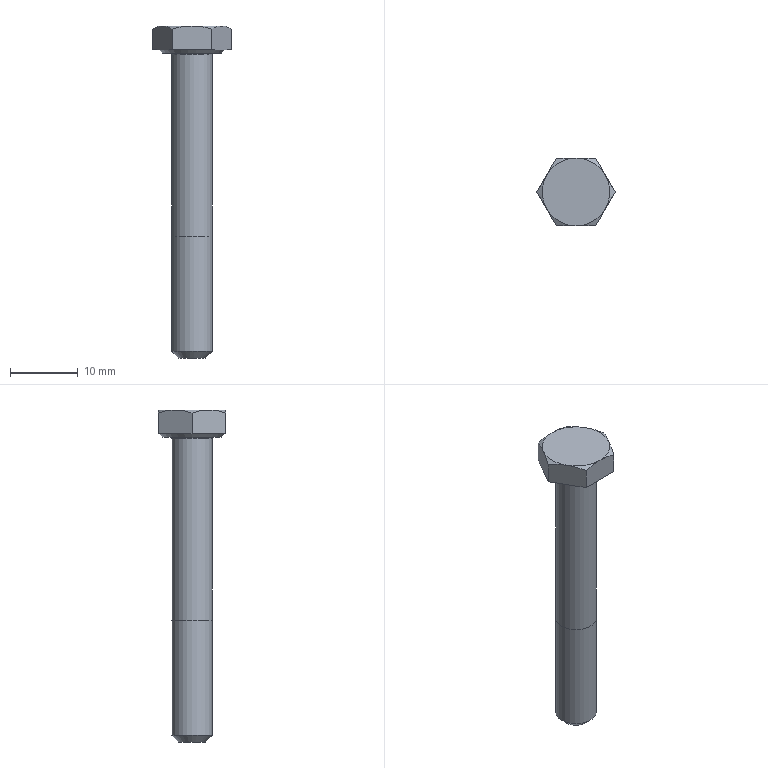Part | NX | features BREP 1, DATUM_CSYS 1 | 1 solid | 21 faces | box 11.547 x 10 x 49 mm | volume 1599 mm3 | plane 10 | cone 8 | cylinder 2 | torus 1 | commonest cylinder face diameters 6 x2
STEP:
#1=CARTESIAN_POINT('',(4.33,2.5,4.));
#2=VERTEX_POINT('',#1);
#3=CARTESIAN_POINT('',(4.33,-2.5,4.));
#4=VERTEX_POINT('',#3);
#5=CARTESIAN_POINT('',(0.,0.,4.));
#6=DIRECTION('',(0.,0.,-1.));
#7=DIRECTION('',(0.866,0.5,0.));
#8=AXIS2_PLACEMENT_3D('',#5,#6,#7);
#9=CIRCLE('',#8,5.);
#10=EDGE_CURVE('',#2,#4,#9,.T.);
#11=ORIENTED_EDGE('',*,*,#10,.F.);
#12=CARTESIAN_POINT('',(0.,5.,4.));
#13=VERTEX_POINT('',#12);
#14=CARTESIAN_POINT('',(0.,0.,4.));
#15=DIRECTION('',(0.,0.,1.));
#16=DIRECTION('',(0.866,0.5,0.));
#17=AXIS2_PLACEMENT_3D('',#14,#15,#16);
#18=CIRCLE('',#17,5.);
#19=EDGE_CURVE('',#2,#13,#18,.T.);
#20=ORIENTED_EDGE('',*,*,#19,.T.);
#21=CARTESIAN_POINT('',(-4.33,2.5,4.));
#22=VERTEX_POINT('',#21);
#23=CARTESIAN_POINT('',(0.,0.,4.));
#24=DIRECTION('',(0.,0.,1.));
#25=DIRECTION('',(0.,1.,0.));
#26=AXIS2_PLACEMENT_3D('',#23,#24,#25);
#27=CIRCLE('',#26,5.);
#28=EDGE_CURVE('',#13,#22,#27,.T.);
#29=ORIENTED_EDGE('',*,*,#28,.T.);
#30=CARTESIAN_POINT('',(-4.33,-2.5,4.));
#31=VERTEX_POINT('',#30);
#32=CARTESIAN_POINT('',(0.,0.,4.));
#33=DIRECTION('',(0.,0.,1.));
#34=DIRECTION('',(-0.866,0.5,0.));
#35=AXIS2_PLACEMENT_3D('',#32,#33,#34);
#36=CIRCLE('',#35,5.);
#37=EDGE_CURVE('',#22,#31,#36,.T.);
#38=ORIENTED_EDGE('',*,*,#37,.T.);
#39=CARTESIAN_POINT('',(0.,-5.,4.));
#40=VERTEX_POINT('',#39);
#41=CARTESIAN_POINT('',(0.,0.,4.));
#42=DIRECTION('',(0.,0.,1.));
#43=DIRECTION('',(-0.866,-0.5,0.));
#44=AXIS2_PLACEMENT_3D('',#41,#42,#43);
#45=CIRCLE('',#44,5.);
#46=EDGE_CURVE('',#31,#40,#45,.T.);
#47=ORIENTED_EDGE('',*,*,#46,.T.);
#48=CARTESIAN_POINT('',(0.,0.,4.));
#49=DIRECTION('',(0.,0.,1.));
#50=DIRECTION('',(0.,-1.,0.));
#51=AXIS2_PLACEMENT_3D('',#48,#49,#50);
#52=CIRCLE('',#51,5.);
#53=EDGE_CURVE('',#40,#4,#52,.T.);
#54=ORIENTED_EDGE('',*,*,#53,.T.);
#55=EDGE_LOOP('',(#11,#20,#29,#38,#47,#54));
#56=FACE_BOUND('',#55,.T.);
#57=CARTESIAN_POINT('',(0.,0.7735,4.));
#58=DIRECTION('',(0.,0.,1.));
#59=DIRECTION('',(-1.,0.,0.));
#60=AXIS2_PLACEMENT_3D('',#57,#58,#59);
#61=PLANE('',#60);
#62=ADVANCED_FACE('',(#56),#61,.T.);
#63=CARTESIAN_POINT('',(5.774,0.,0.5));
#64=VERTEX_POINT('',#63);
#65=CARTESIAN_POINT('',(2.887,5.,0.5));
#66=VERTEX_POINT('',#65);
#67=CARTESIAN_POINT('',(5.774,0.,0.5));
#68=DIRECTION('',(-0.5,0.866,0.));
#69=VECTOR('',#68,1000.);
#70=LINE('',#67,#69);
#71=EDGE_CURVE('',#64,#66,#70,.T.);
#72=ORIENTED_EDGE('',*,*,#71,.T.);
#73=CARTESIAN_POINT('',(2.887,5.,3.553));
#74=VERTEX_POINT('',#73);
#75=CARTESIAN_POINT('',(2.887,5.,0.5));
#76=DIRECTION('',(0.,0.,1.));
#77=VECTOR('',#76,1000.);
#78=LINE('',#75,#77);
#79=EDGE_CURVE('',#66,#74,#78,.T.);
#80=ORIENTED_EDGE('',*,*,#79,.T.);
#81=CARTESIAN_POINT('',(4.33,2.5,4.));
#82=CARTESIAN_POINT('',(3.66,3.66,4.));
#83=CARTESIAN_POINT('',(2.887,5.,3.553));
#84=(BOUNDED_CURVE()B_SPLINE_CURVE(2,(#81,#82,#83),.UNSPECIFIED.,.F.,.F.)B_SPLINE_CURVE_WITH_KNOTS((3,3),(0.,1.),.PIECEWISE_BEZIER_KNOTS.)CURVE()GEOMETRIC_REPRESENTATION_ITEM()RATIONAL_B_SPLINE_CURVE((1.444,1.444,1.34))REPRESENTATION_ITEM(''));
#85=EDGE_CURVE('',#2,#74,#84,.T.);
#86=ORIENTED_EDGE('',*,*,#85,.F.);
#87=CARTESIAN_POINT('',(5.774,0.,3.553));
#88=VERTEX_POINT('',#87);
#89=CARTESIAN_POINT('',(5.774,0.,3.553));
#90=CARTESIAN_POINT('',(5.,1.34,4.));
#91=CARTESIAN_POINT('',(4.33,2.5,4.));
#92=(BOUNDED_CURVE()B_SPLINE_CURVE(2,(#89,#90,#91),.UNSPECIFIED.,.F.,.F.)B_SPLINE_CURVE_WITH_KNOTS((3,3),(0.,1.),.PIECEWISE_BEZIER_KNOTS.)CURVE()GEOMETRIC_REPRESENTATION_ITEM()RATIONAL_B_SPLINE_CURVE((1.34,1.444,1.444))REPRESENTATION_ITEM(''));
#93=EDGE_CURVE('',#88,#2,#92,.T.);
#94=ORIENTED_EDGE('',*,*,#93,.F.);
#95=CARTESIAN_POINT('',(5.774,0.,0.5));
#96=DIRECTION('',(0.,0.,1.));
#97=VECTOR('',#96,1000.);
#98=LINE('',#95,#97);
#99=EDGE_CURVE('',#64,#88,#98,.T.);
#100=ORIENTED_EDGE('',*,*,#99,.F.);
#101=EDGE_LOOP('',(#72,#80,#86,#94,#100));
#102=FACE_BOUND('',#101,.T.);
#103=CARTESIAN_POINT('',(4.33,2.5,2.25));
#104=DIRECTION('',(0.866,0.5,0.));
#105=DIRECTION('',(0.5,-0.866,0.));
#106=AXIS2_PLACEMENT_3D('',#103,#104,#105);
#107=PLANE('',#106);
#108=ADVANCED_FACE('',(#102),#107,.T.);
#109=CARTESIAN_POINT('',(-2.887,5.,0.5));
#110=VERTEX_POINT('',#109);
#111=CARTESIAN_POINT('',(2.887,5.,0.5));
#112=DIRECTION('',(-1.,0.,0.));
#113=VECTOR('',#112,1000.);
#114=LINE('',#111,#113);
#115=EDGE_CURVE('',#66,#110,#114,.T.);
#116=ORIENTED_EDGE('',*,*,#115,.T.);
#117=CARTESIAN_POINT('',(-2.887,5.,3.553));
#118=VERTEX_POINT('',#117);
#119=CARTESIAN_POINT('',(-2.887,5.,0.5));
#120=DIRECTION('',(0.,0.,1.));
#121=VECTOR('',#120,1000.);
#122=LINE('',#119,#121);
#123=EDGE_CURVE('',#110,#118,#122,.T.);
#124=ORIENTED_EDGE('',*,*,#123,.T.);
#125=CARTESIAN_POINT('',(0.,5.,4.));
#126=CARTESIAN_POINT('',(-1.34,5.,4.));
#127=CARTESIAN_POINT('',(-2.887,5.,3.553));
#128=(BOUNDED_CURVE()B_SPLINE_CURVE(2,(#125,#126,#127),.UNSPECIFIED.,.F.,.F.)B_SPLINE_CURVE_WITH_KNOTS((3,3),(0.,1.),.PIECEWISE_BEZIER_KNOTS.)CURVE()GEOMETRIC_REPRESENTATION_ITEM()RATIONAL_B_SPLINE_CURVE((1.444,1.444,1.34))REPRESENTATION_ITEM(''));
#129=EDGE_CURVE('',#13,#118,#128,.T.);
#130=ORIENTED_EDGE('',*,*,#129,.F.);
#131=CARTESIAN_POINT('',(2.887,5.,3.553));
#132=CARTESIAN_POINT('',(1.34,5.,4.));
#133=CARTESIAN_POINT('',(0.,5.,4.));
#134=(BOUNDED_CURVE()B_SPLINE_CURVE(2,(#131,#132,#133),.UNSPECIFIED.,.F.,.F.)B_SPLINE_CURVE_WITH_KNOTS((3,3),(0.,1.),.PIECEWISE_BEZIER_KNOTS.)CURVE()GEOMETRIC_REPRESENTATION_ITEM()RATIONAL_B_SPLINE_CURVE((1.34,1.444,1.444))REPRESENTATION_ITEM(''));
#135=EDGE_CURVE('',#74,#13,#134,.T.);
#136=ORIENTED_EDGE('',*,*,#135,.F.);
#137=ORIENTED_EDGE('',*,*,#79,.F.);
#138=EDGE_LOOP('',(#116,#124,#130,#136,#137));
#139=FACE_BOUND('',#138,.T.);
#140=CARTESIAN_POINT('',(0.,5.,2.25));
#141=DIRECTION('',(0.,1.,0.));
#142=DIRECTION('',(1.,0.,0.));
#143=AXIS2_PLACEMENT_3D('',#140,#141,#142);
#144=PLANE('',#143);
#145=ADVANCED_FACE('',(#139),#144,.T.);
#146=CARTESIAN_POINT('',(-5.774,0.,0.5));
#147=VERTEX_POINT('',#146);
#148=CARTESIAN_POINT('',(-2.887,5.,0.5));
#149=DIRECTION('',(-0.5,-0.866,0.));
#150=VECTOR('',#149,1000.);
#151=LINE('',#148,#150);
#152=EDGE_CURVE('',#110,#147,#151,.T.);
#153=ORIENTED_EDGE('',*,*,#152,.T.);
#154=CARTESIAN_POINT('',(-5.774,0.,3.553));
#155=VERTEX_POINT('',#154);
#156=CARTESIAN_POINT('',(-5.774,0.,0.5));
#157=DIRECTION('',(0.,0.,1.));
#158=VECTOR('',#157,1000.);
#159=LINE('',#156,#158);
#160=EDGE_CURVE('',#147,#155,#159,.T.);
#161=ORIENTED_EDGE('',*,*,#160,.T.);
#162=CARTESIAN_POINT('',(-4.33,2.5,4.));
#163=CARTESIAN_POINT('',(-5.,1.34,4.));
#164=CARTESIAN_POINT('',(-5.774,0.,3.553));
#165=(BOUNDED_CURVE()B_SPLINE_CURVE(2,(#162,#163,#164),.UNSPECIFIED.,.F.,.F.)B_SPLINE_CURVE_WITH_KNOTS((3,3),(0.,1.),.PIECEWISE_BEZIER_KNOTS.)CURVE()GEOMETRIC_REPRESENTATION_ITEM()RATIONAL_B_SPLINE_CURVE((1.444,1.444,1.34))REPRESENTATION_ITEM(''));
#166=EDGE_CURVE('',#22,#155,#165,.T.);
#167=ORIENTED_EDGE('',*,*,#166,.F.);
#168=CARTESIAN_POINT('',(-2.887,5.,3.553));
#169=CARTESIAN_POINT('',(-3.66,3.66,4.));
#170=CARTESIAN_POINT('',(-4.33,2.5,4.));
#171=(BOUNDED_CURVE()B_SPLINE_CURVE(2,(#168,#169,#170),.UNSPECIFIED.,.F.,.F.)B_SPLINE_CURVE_WITH_KNOTS((3,3),(0.,1.),.PIECEWISE_BEZIER_KNOTS.)CURVE()GEOMETRIC_REPRESENTATION_ITEM()RATIONAL_B_SPLINE_CURVE((1.34,1.444,1.444))REPRESENTATION_ITEM(''));
#172=EDGE_CURVE('',#118,#22,#171,.T.);
#173=ORIENTED_EDGE('',*,*,#172,.F.);
#174=ORIENTED_EDGE('',*,*,#123,.F.);
#175=EDGE_LOOP('',(#153,#161,#167,#173,#174));
#176=FACE_BOUND('',#175,.T.);
#177=CARTESIAN_POINT('',(-4.33,2.5,2.25));
#178=DIRECTION('',(-0.866,0.5,0.));
#179=DIRECTION('',(0.5,0.866,0.));
#180=AXIS2_PLACEMENT_3D('',#177,#178,#179);
#181=PLANE('',#180);
#182=ADVANCED_FACE('',(#176),#181,.T.);
#183=CARTESIAN_POINT('',(-2.887,-5.,0.5));
#184=VERTEX_POINT('',#183);
#185=CARTESIAN_POINT('',(-5.774,0.,0.5));
#186=DIRECTION('',(0.5,-0.866,0.));
#187=VECTOR('',#186,1000.);
#188=LINE('',#185,#187);
#189=EDGE_CURVE('',#147,#184,#188,.T.);
#190=ORIENTED_EDGE('',*,*,#189,.T.);
#191=CARTESIAN_POINT('',(-2.887,-5.,3.553));
#192=VERTEX_POINT('',#191);
#193=CARTESIAN_POINT('',(-2.887,-5.,0.5));
#194=DIRECTION('',(0.,0.,1.));
#195=VECTOR('',#194,1000.);
#196=LINE('',#193,#195);
#197=EDGE_CURVE('',#184,#192,#196,.T.);
#198=ORIENTED_EDGE('',*,*,#197,.T.);
#199=CARTESIAN_POINT('',(-4.33,-2.5,4.));
#200=CARTESIAN_POINT('',(-3.66,-3.66,4.));
#201=CARTESIAN_POINT('',(-2.887,-5.,3.553));
#202=(BOUNDED_CURVE()B_SPLINE_CURVE(2,(#199,#200,#201),.UNSPECIFIED.,.F.,.F.)B_SPLINE_CURVE_WITH_KNOTS((3,3),(0.,1.),.PIECEWISE_BEZIER_KNOTS.)CURVE()GEOMETRIC_REPRESENTATION_ITEM()RATIONAL_B_SPLINE_CURVE((1.444,1.444,1.34))REPRESENTATION_ITEM(''));
#203=EDGE_CURVE('',#31,#192,#202,.T.);
#204=ORIENTED_EDGE('',*,*,#203,.F.);
#205=CARTESIAN_POINT('',(-5.774,0.,3.553));
#206=CARTESIAN_POINT('',(-5.,-1.34,4.));
#207=CARTESIAN_POINT('',(-4.33,-2.5,4.));
#208=(BOUNDED_CURVE()B_SPLINE_CURVE(2,(#205,#206,#207),.UNSPECIFIED.,.F.,.F.)B_SPLINE_CURVE_WITH_KNOTS((3,3),(0.,1.),.PIECEWISE_BEZIER_KNOTS.)CURVE()GEOMETRIC_REPRESENTATION_ITEM()RATIONAL_B_SPLINE_CURVE((1.34,1.444,1.444))REPRESENTATION_ITEM(''));
#209=EDGE_CURVE('',#155,#31,#208,.T.);
#210=ORIENTED_EDGE('',*,*,#209,.F.);
#211=ORIENTED_EDGE('',*,*,#160,.F.);
#212=EDGE_LOOP('',(#190,#198,#204,#210,#211));
#213=FACE_BOUND('',#212,.T.);
#214=CARTESIAN_POINT('',(-4.33,-2.5,2.25));
#215=DIRECTION('',(-0.866,-0.5,0.));
#216=DIRECTION('',(-0.5,0.866,0.));
#217=AXIS2_PLACEMENT_3D('',#214,#215,#216);
#218=PLANE('',#217);
#219=ADVANCED_FACE('',(#213),#218,.T.);
#220=CARTESIAN_POINT('',(2.887,-5.,0.5));
#221=VERTEX_POINT('',#220);
#222=CARTESIAN_POINT('',(-2.887,-5.,0.5));
#223=DIRECTION('',(1.,0.,0.));
#224=VECTOR('',#223,1000.);
#225=LINE('',#222,#224);
#226=EDGE_CURVE('',#184,#221,#225,.T.);
#227=ORIENTED_EDGE('',*,*,#226,.T.);
#228=CARTESIAN_POINT('',(2.887,-5.,3.553));
#229=VERTEX_POINT('',#228);
#230=CARTESIAN_POINT('',(2.887,-5.,0.5));
#231=DIRECTION('',(0.,0.,1.));
#232=VECTOR('',#231,1000.);
#233=LINE('',#230,#232);
#234=EDGE_CURVE('',#221,#229,#233,.T.);
#235=ORIENTED_EDGE('',*,*,#234,.T.);
#236=CARTESIAN_POINT('',(0.,-5.,4.));
#237=CARTESIAN_POINT('',(1.34,-5.,4.));
#238=CARTESIAN_POINT('',(2.887,-5.,3.553));
#239=(BOUNDED_CURVE()B_SPLINE_CURVE(2,(#236,#237,#238),.UNSPECIFIED.,.F.,.F.)B_SPLINE_CURVE_WITH_KNOTS((3,3),(0.,1.),.PIECEWISE_BEZIER_KNOTS.)CURVE()GEOMETRIC_REPRESENTATION_ITEM()RATIONAL_B_SPLINE_CURVE((1.444,1.444,1.34))REPRESENTATION_ITEM(''));
#240=EDGE_CURVE('',#40,#229,#239,.T.);
#241=ORIENTED_EDGE('',*,*,#240,.F.);
#242=CARTESIAN_POINT('',(-2.887,-5.,3.553));
#243=CARTESIAN_POINT('',(-1.34,-5.,4.));
#244=CARTESIAN_POINT('',(0.,-5.,4.));
#245=(BOUNDED_CURVE()B_SPLINE_CURVE(2,(#242,#243,#244),.UNSPECIFIED.,.F.,.F.)B_SPLINE_CURVE_WITH_KNOTS((3,3),(0.,1.),.PIECEWISE_BEZIER_KNOTS.)CURVE()GEOMETRIC_REPRESENTATION_ITEM()RATIONAL_B_SPLINE_CURVE((1.34,1.444,1.444))REPRESENTATION_ITEM(''));
#246=EDGE_CURVE('',#192,#40,#245,.T.);
#247=ORIENTED_EDGE('',*,*,#246,.F.);
#248=ORIENTED_EDGE('',*,*,#197,.F.);
#249=EDGE_LOOP('',(#227,#235,#241,#247,#248));
#250=FACE_BOUND('',#249,.T.);
#251=CARTESIAN_POINT('',(0.,-5.,2.25));
#252=DIRECTION('',(0.,-1.,0.));
#253=DIRECTION('',(-1.,0.,0.));
#254=AXIS2_PLACEMENT_3D('',#251,#252,#253);
#255=PLANE('',#254);
#256=ADVANCED_FACE('',(#250),#255,.T.);
#257=CARTESIAN_POINT('',(2.887,-5.,0.5));
#258=DIRECTION('',(0.5,0.866,0.));
#259=VECTOR('',#258,1000.);
#260=LINE('',#257,#259);
#261=EDGE_CURVE('',#221,#64,#260,.T.);
#262=ORIENTED_EDGE('',*,*,#261,.T.);
#263=ORIENTED_EDGE('',*,*,#99,.T.);
#264=CARTESIAN_POINT('',(4.33,-2.5,4.));
#265=CARTESIAN_POINT('',(5.,-1.34,4.));
#266=CARTESIAN_POINT('',(5.774,0.,3.553));
#267=(BOUNDED_CURVE()B_SPLINE_CURVE(2,(#264,#265,#266),.UNSPECIFIED.,.F.,.F.)B_SPLINE_CURVE_WITH_KNOTS((3,3),(0.,1.),.PIECEWISE_BEZIER_KNOTS.)CURVE()GEOMETRIC_REPRESENTATION_ITEM()RATIONAL_B_SPLINE_CURVE((1.444,1.444,1.34))REPRESENTATION_ITEM(''));
#268=EDGE_CURVE('',#4,#88,#267,.T.);
#269=ORIENTED_EDGE('',*,*,#268,.F.);
#270=CARTESIAN_POINT('',(2.887,-5.,3.553));
#271=CARTESIAN_POINT('',(3.66,-3.66,4.));
#272=CARTESIAN_POINT('',(4.33,-2.5,4.));
#273=(BOUNDED_CURVE()B_SPLINE_CURVE(2,(#270,#271,#272),.UNSPECIFIED.,.F.,.F.)B_SPLINE_CURVE_WITH_KNOTS((3,3),(0.,1.),.PIECEWISE_BEZIER_KNOTS.)CURVE()GEOMETRIC_REPRESENTATION_ITEM()RATIONAL_B_SPLINE_CURVE((1.34,1.444,1.444))REPRESENTATION_ITEM(''));
#274=EDGE_CURVE('',#229,#4,#273,.T.);
#275=ORIENTED_EDGE('',*,*,#274,.F.);
#276=ORIENTED_EDGE('',*,*,#234,.F.);
#277=EDGE_LOOP('',(#262,#263,#269,#275,#276));
#278=FACE_BOUND('',#277,.T.);
#279=CARTESIAN_POINT('',(4.33,-2.5,2.25));
#280=DIRECTION('',(0.866,-0.5,0.));
#281=DIRECTION('',(-0.5,-0.866,0.));
#282=AXIS2_PLACEMENT_3D('',#279,#280,#281);
#283=PLANE('',#282);
#284=ADVANCED_FACE('',(#278),#283,.T.);
#285=ORIENTED_EDGE('',*,*,#261,.F.);
#286=ORIENTED_EDGE('',*,*,#226,.F.);
#287=ORIENTED_EDGE('',*,*,#189,.F.);
#288=ORIENTED_EDGE('',*,*,#152,.F.);
#289=ORIENTED_EDGE('',*,*,#115,.F.);
#290=ORIENTED_EDGE('',*,*,#71,.F.);
#291=EDGE_LOOP('',(#285,#286,#287,#288,#289,#290));
#292=FACE_BOUND('',#291,.T.);
#293=CARTESIAN_POINT('',(4.84,0.,0.5));
#294=VERTEX_POINT('',#293);
#295=CARTESIAN_POINT('',(0.,0.,0.5));
#296=DIRECTION('',(0.,0.,1.));
#297=DIRECTION('',(1.,0.,0.));
#298=AXIS2_PLACEMENT_3D('',#295,#296,#297);
#299=CIRCLE('',#298,4.84);
#300=EDGE_CURVE('',#294,#294,#299,.T.);
#301=ORIENTED_EDGE('',*,*,#300,.T.);
#302=EDGE_LOOP('',(#301));
#303=FACE_BOUND('',#302,.T.);
#304=CARTESIAN_POINT('',(0.,0.7735,0.5));
#305=DIRECTION('',(0.,0.,1.));
#306=DIRECTION('',(-1.,0.,0.));
#307=AXIS2_PLACEMENT_3D('',#304,#305,#306);
#308=PLANE('',#307);
#309=ADVANCED_FACE('',(#292,#303),#308,.F.);
#310=CARTESIAN_POINT('',(4.34,0.,0.));
#311=VERTEX_POINT('',#310);
#312=CARTESIAN_POINT('',(0.,0.,0.));
#313=DIRECTION('',(0.,0.,1.));
#314=DIRECTION('',(1.,0.,0.));
#315=AXIS2_PLACEMENT_3D('',#312,#313,#314);
#316=CIRCLE('',#315,4.34);
#317=EDGE_CURVE('',#311,#311,#316,.T.);
#318=ORIENTED_EDGE('',*,*,#317,.T.);
#319=CARTESIAN_POINT('',(4.34,0.,0.));
#320=DIRECTION('',(0.7071,0.,0.7071));
#321=VECTOR('',#320,1000.);
#322=LINE('',#319,#321);
#323=EDGE_CURVE('',#311,#294,#322,.T.);
#324=ORIENTED_EDGE('',*,*,#323,.T.);
#325=ORIENTED_EDGE('',*,*,#300,.F.);
#326=ORIENTED_EDGE('',*,*,#323,.F.);
#327=EDGE_LOOP('',(#318,#324,#325,#326));
#328=FACE_BOUND('',#327,.T.);
#329=CARTESIAN_POINT('',(0.,0.,0.));
#330=DIRECTION('',(0.,0.,1.));
#331=DIRECTION('',(-1.,0.,0.));
#332=AXIS2_PLACEMENT_3D('',#329,#330,#331);
#333=CONICAL_SURFACE('',#332,4.34,0.7854);
#334=ADVANCED_FACE('',(#328),#333,.T.);
#335=ORIENTED_EDGE('',*,*,#317,.F.);
#336=EDGE_LOOP('',(#335));
#337=FACE_BOUND('',#336,.T.);
#338=CARTESIAN_POINT('',(3.25,0.,0.));
#339=VERTEX_POINT('',#338);
#340=CARTESIAN_POINT('',(0.,0.,0.));
#341=DIRECTION('',(0.,0.,1.));
#342=DIRECTION('',(1.,0.,0.));
#343=AXIS2_PLACEMENT_3D('',#340,#341,#342);
#344=CIRCLE('',#343,3.25);
#345=EDGE_CURVE('',#339,#339,#344,.T.);
#346=ORIENTED_EDGE('',*,*,#345,.T.);
#347=EDGE_LOOP('',(#346));
#348=FACE_BOUND('',#347,.T.);
#349=CARTESIAN_POINT('',(0.,0.,0.));
#350=DIRECTION('',(0.,0.,1.));
#351=DIRECTION('',(-1.,0.,0.));
#352=AXIS2_PLACEMENT_3D('',#349,#350,#351);
#353=PLANE('',#352);
#354=ADVANCED_FACE('',(#337,#348),#353,.F.);
#355=CARTESIAN_POINT('',(3.,0.,-0.25));
#356=VERTEX_POINT('',#355);
#357=CARTESIAN_POINT('',(0.,0.,-0.25));
#358=DIRECTION('',(0.,0.,1.));
#359=DIRECTION('',(1.,0.,0.));
#360=AXIS2_PLACEMENT_3D('',#357,#358,#359);
#361=CIRCLE('',#360,3.);
#362=EDGE_CURVE('',#356,#356,#361,.T.);
#363=ORIENTED_EDGE('',*,*,#362,.T.);
#364=CARTESIAN_POINT('',(3.25,0.,-0.25));
#365=DIRECTION('',(0.,1.,0.));
#366=DIRECTION('',(-1.,0.,0.));
#367=AXIS2_PLACEMENT_3D('',#364,#365,#366);
#368=CIRCLE('',#367,0.25);
#369=EDGE_CURVE('',#356,#339,#368,.T.);
#370=ORIENTED_EDGE('',*,*,#369,.T.);
#371=ORIENTED_EDGE('',*,*,#345,.F.);
#372=ORIENTED_EDGE('',*,*,#369,.F.);
#373=EDGE_LOOP('',(#363,#370,#371,#372));
#374=FACE_BOUND('',#373,.T.);
#375=CARTESIAN_POINT('',(0.,0.,-0.25));
#376=DIRECTION('',(0.,0.,-1.));
#377=DIRECTION('',(-1.,0.,0.));
#378=AXIS2_PLACEMENT_3D('',#375,#376,#377);
#379=TOROIDAL_SURFACE('',#378,3.25,0.25);
#380=ADVANCED_FACE('',(#374),#379,.F.);
#381=CARTESIAN_POINT('',(3.,0.,-27.));
#382=VERTEX_POINT('',#381);
#383=CARTESIAN_POINT('',(0.,0.,-27.));
#384=DIRECTION('',(0.,0.,1.));
#385=DIRECTION('',(1.,0.,0.));
#386=AXIS2_PLACEMENT_3D('',#383,#384,#385);
#387=CIRCLE('',#386,3.);
#388=EDGE_CURVE('',#382,#382,#387,.T.);
#389=ORIENTED_EDGE('',*,*,#388,.T.);
#390=CARTESIAN_POINT('',(3.,0.,-27.));
#391=DIRECTION('',(0.,0.,1.));
#392=VECTOR('',#391,1000.);
#393=LINE('',#390,#392);
#394=EDGE_CURVE('',#382,#356,#393,.T.);
#395=ORIENTED_EDGE('',*,*,#394,.T.);
#396=ORIENTED_EDGE('',*,*,#362,.F.);
#397=ORIENTED_EDGE('',*,*,#394,.F.);
#398=EDGE_LOOP('',(#389,#395,#396,#397));
#399=FACE_BOUND('',#398,.T.);
#400=CARTESIAN_POINT('',(0.,0.,-27.));
#401=DIRECTION('',(0.,0.,1.));
#402=DIRECTION('',(-1.,0.,0.));
#403=AXIS2_PLACEMENT_3D('',#400,#401,#402);
#404=CYLINDRICAL_SURFACE('',#403,3.);
#405=ADVANCED_FACE('',(#399),#404,.T.);
#406=CARTESIAN_POINT('',(3.,0.,-44.));
#407=VERTEX_POINT('',#406);
#408=CARTESIAN_POINT('',(0.,0.,-44.));
#409=DIRECTION('',(0.,0.,1.));
#410=DIRECTION('',(1.,0.,0.));
#411=AXIS2_PLACEMENT_3D('',#408,#409,#410);
#412=CIRCLE('',#411,3.);
#413=EDGE_CURVE('',#407,#407,#412,.T.);
#414=ORIENTED_EDGE('',*,*,#413,.T.);
#415=CARTESIAN_POINT('',(3.,0.,-44.));
#416=DIRECTION('',(0.,0.,1.));
#417=VECTOR('',#416,1000.);
#418=LINE('',#415,#417);
#419=EDGE_CURVE('',#407,#382,#418,.T.);
#420=ORIENTED_EDGE('',*,*,#419,.T.);
#421=ORIENTED_EDGE('',*,*,#388,.F.);
#422=ORIENTED_EDGE('',*,*,#419,.F.);
#423=EDGE_LOOP('',(#414,#420,#421,#422));
#424=FACE_BOUND('',#423,.T.);
#425=CARTESIAN_POINT('',(0.,0.,-44.));
#426=DIRECTION('',(0.,0.,1.));
#427=DIRECTION('',(-1.,0.,0.));
#428=AXIS2_PLACEMENT_3D('',#425,#426,#427);
#429=CYLINDRICAL_SURFACE('',#428,3.);
#430=ADVANCED_FACE('',(#424),#429,.T.);
#431=CARTESIAN_POINT('',(2.,0.,-45.));
#432=VERTEX_POINT('',#431);
#433=CARTESIAN_POINT('',(0.,0.,-45.));
#434=DIRECTION('',(0.,0.,1.));
#435=DIRECTION('',(1.,0.,0.));
#436=AXIS2_PLACEMENT_3D('',#433,#434,#435);
#437=CIRCLE('',#436,2.);
#438=EDGE_CURVE('',#432,#432,#437,.T.);
#439=ORIENTED_EDGE('',*,*,#438,.T.);
#440=CARTESIAN_POINT('',(2.,0.,-45.));
#441=DIRECTION('',(0.7071,0.,0.7071));
#442=VECTOR('',#441,1000.);
#443=LINE('',#440,#442);
#444=EDGE_CURVE('',#432,#407,#443,.T.);
#445=ORIENTED_EDGE('',*,*,#444,.T.);
#446=ORIENTED_EDGE('',*,*,#413,.F.);
#447=ORIENTED_EDGE('',*,*,#444,.F.);
#448=EDGE_LOOP('',(#439,#445,#446,#447));
#449=FACE_BOUND('',#448,.T.);
#450=CARTESIAN_POINT('',(0.,0.,-45.));
#451=DIRECTION('',(0.,0.,1.));
#452=DIRECTION('',(-1.,0.,0.));
#453=AXIS2_PLACEMENT_3D('',#450,#451,#452);
#454=CONICAL_SURFACE('',#453,2.,0.7854);
#455=ADVANCED_FACE('',(#449),#454,.T.);
#456=ORIENTED_EDGE('',*,*,#438,.F.);
#457=EDGE_LOOP('',(#456));
#458=FACE_BOUND('',#457,.T.);
#459=CARTESIAN_POINT('',(0.,0.,-45.));
#460=DIRECTION('',(0.,0.,1.));
#461=DIRECTION('',(-1.,0.,0.));
#462=AXIS2_PLACEMENT_3D('',#459,#460,#461);
#463=PLANE('',#462);
#464=ADVANCED_FACE('',(#458),#463,.F.);
#465=ORIENTED_EDGE('',*,*,#19,.F.);
#466=ORIENTED_EDGE('',*,*,#85,.T.);
#467=ORIENTED_EDGE('',*,*,#135,.T.);
#468=EDGE_LOOP('',(#465,#466,#467));
#469=FACE_BOUND('',#468,.T.);
#470=CARTESIAN_POINT('',(0.,0.,4.));
#471=DIRECTION('',(0.,0.,-1.));
#472=DIRECTION('',(-0.922,-0.3873,0.));
#473=AXIS2_PLACEMENT_3D('',#470,#471,#472);
#474=CONICAL_SURFACE('',#473,5.,1.047);
#475=ADVANCED_FACE('',(#469),#474,.T.);
#476=ORIENTED_EDGE('',*,*,#93,.T.);
#477=ORIENTED_EDGE('',*,*,#10,.T.);
#478=ORIENTED_EDGE('',*,*,#268,.T.);
#479=EDGE_LOOP('',(#476,#477,#478));
#480=FACE_BOUND('',#479,.T.);
#481=CARTESIAN_POINT('',(0.,0.,4.));
#482=DIRECTION('',(0.,0.,-1.));
#483=DIRECTION('',(-0.866,0.5,0.));
#484=AXIS2_PLACEMENT_3D('',#481,#482,#483);
#485=CONICAL_SURFACE('',#484,5.,1.047);
#486=ADVANCED_FACE('',(#480),#485,.T.);
#487=ORIENTED_EDGE('',*,*,#28,.F.);
#488=ORIENTED_EDGE('',*,*,#129,.T.);
#489=ORIENTED_EDGE('',*,*,#172,.T.);
#490=EDGE_LOOP('',(#487,#488,#489));
#491=FACE_BOUND('',#490,.T.);
#492=CARTESIAN_POINT('',(0.,0.,4.));
#493=DIRECTION('',(0.,0.,-1.));
#494=DIRECTION('',(-0.922,-0.3873,0.));
#495=AXIS2_PLACEMENT_3D('',#492,#493,#494);
#496=CONICAL_SURFACE('',#495,5.,1.047);
#497=ADVANCED_FACE('',(#491),#496,.T.);
#498=ORIENTED_EDGE('',*,*,#37,.F.);
#499=ORIENTED_EDGE('',*,*,#166,.T.);
#500=ORIENTED_EDGE('',*,*,#209,.T.);
#501=EDGE_LOOP('',(#498,#499,#500));
#502=FACE_BOUND('',#501,.T.);
#503=CARTESIAN_POINT('',(0.,0.,4.));
#504=DIRECTION('',(0.,0.,-1.));
#505=DIRECTION('',(-0.922,-0.3873,0.));
#506=AXIS2_PLACEMENT_3D('',#503,#504,#505);
#507=CONICAL_SURFACE('',#506,5.,1.047);
#508=ADVANCED_FACE('',(#502),#507,.T.);
#509=ORIENTED_EDGE('',*,*,#46,.F.);
#510=ORIENTED_EDGE('',*,*,#203,.T.);
#511=ORIENTED_EDGE('',*,*,#246,.T.);
#512=EDGE_LOOP('',(#509,#510,#511));
#513=FACE_BOUND('',#512,.T.);
#514=CARTESIAN_POINT('',(0.,0.,4.));
#515=DIRECTION('',(0.,0.,-1.));
#516=DIRECTION('',(-0.922,-0.3873,0.));
#517=AXIS2_PLACEMENT_3D('',#514,#515,#516);
#518=CONICAL_SURFACE('',#517,5.,1.047);
#519=ADVANCED_FACE('',(#513),#518,.T.);
#520=ORIENTED_EDGE('',*,*,#53,.F.);
#521=ORIENTED_EDGE('',*,*,#240,.T.);
#522=ORIENTED_EDGE('',*,*,#274,.T.);
#523=EDGE_LOOP('',(#520,#521,#522));
#524=FACE_BOUND('',#523,.T.);
#525=CARTESIAN_POINT('',(0.,0.,4.));
#526=DIRECTION('',(0.,0.,-1.));
#527=DIRECTION('',(-0.922,-0.3873,0.));
#528=AXIS2_PLACEMENT_3D('',#525,#526,#527);
#529=CONICAL_SURFACE('',#528,5.,1.047);
#530=ADVANCED_FACE('',(#524),#529,.T.);
#531=CLOSED_SHELL('',(#62,#108,#145,#182,#219,#256,#284,#309,#334,#354,#380,#405,#430,#455,#464,#475,#486,#497,#508,#519,#530));
#532=MANIFOLD_SOLID_BREP('',#531);
#533=(LENGTH_UNIT()NAMED_UNIT(*)SI_UNIT(.MILLI.,.METRE.));
#534=UNCERTAINTY_MEASURE_WITH_UNIT(LENGTH_MEASURE(0.00001),#533,'','');
#535=(NAMED_UNIT(*)PLANE_ANGLE_UNIT()SI_UNIT($,.RADIAN.));
#536=(NAMED_UNIT(*)SI_UNIT($,.STERADIAN.)SOLID_ANGLE_UNIT());
#537=(GEOMETRIC_REPRESENTATION_CONTEXT(3)GLOBAL_UNCERTAINTY_ASSIGNED_CONTEXT((#534))GLOBAL_UNIT_ASSIGNED_CONTEXT((#533,#535,#536))REPRESENTATION_CONTEXT('',''));
#538=ADVANCED_BREP_SHAPE_REPRESENTATION('',(#532),#537);